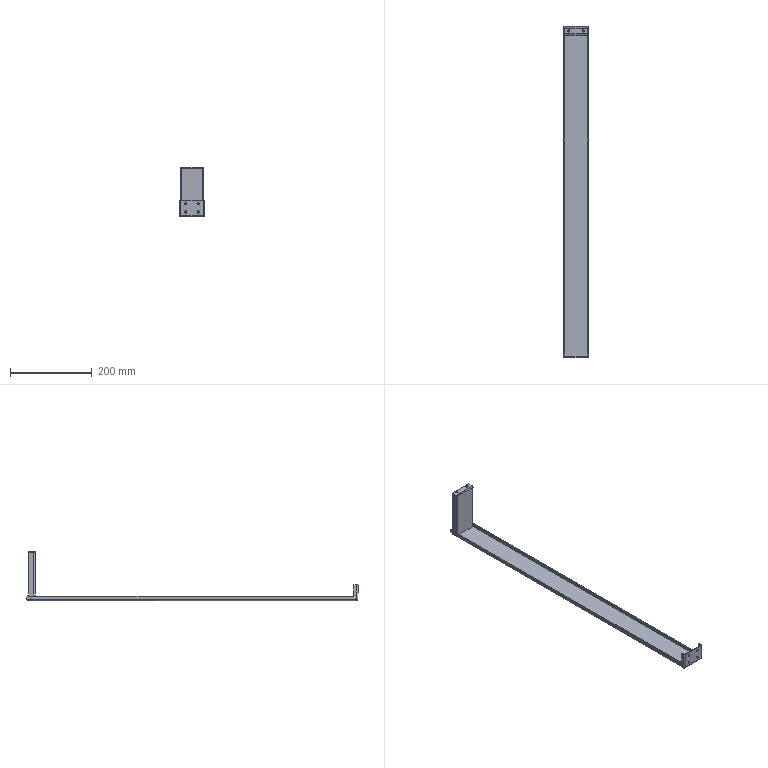Part | SolidWorks | features EdgeFlange 5, FlatPattern 2, ICE 2, SMBaseFlange 2, SheetMetal 2 | 2 solids | 122 faces | box 60 x 812.195 x 122 mm | volume 146456 mm3 | plane 80 | cylinder 34 | spline 8 | commonest cylinder face diameters 5.5 x12 1.473 x11 5.473 x11